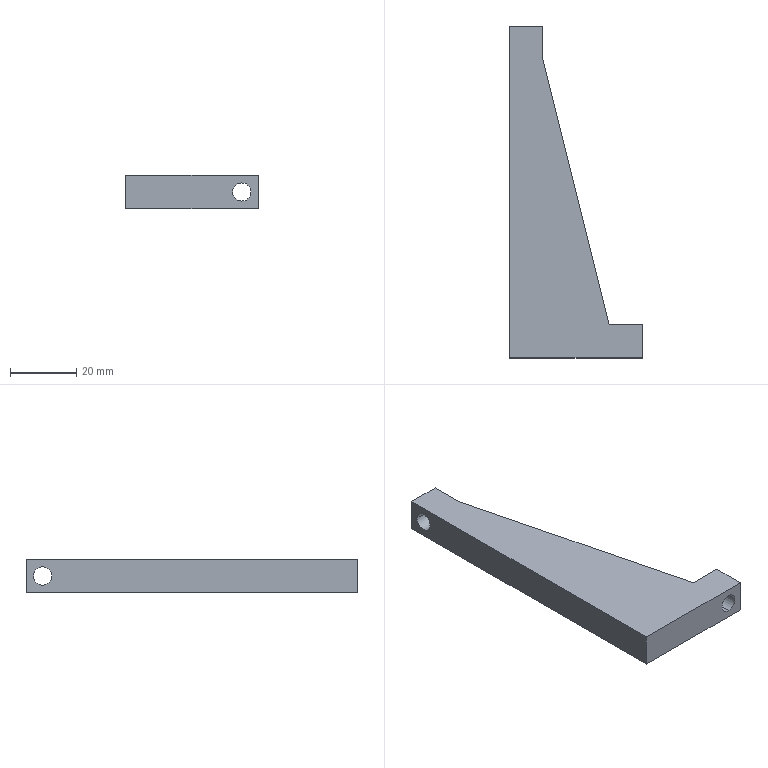Part | STEP file | B06 | 1 solid | 13 faces | box 40 x 100 x 10 mm | volume 20525 mm3 | plane 9 | cylinder 4 | commonest cylinder face diameters 5.5 x4
STEP:
#1=CARTESIAN_POINT('',(0.,0.,0.));
#2=DIRECTION('',(0.,0.,1.));
#3=DIRECTION('',(1.,0.,0.));
#4=AXIS2_PLACEMENT_3D('',#1,#2,#3);
#5=CARTESIAN_POINT('',(15.,-50.,7.75));
#6=VERTEX_POINT('',#5);
#7=CARTESIAN_POINT('',(15.,-40.,7.75));
#8=VERTEX_POINT('',#7);
#9=CARTESIAN_POINT('',(15.,-50.,7.75));
#10=DIRECTION('',(0.,1.,0.));
#11=VECTOR('',#10,1.);
#12=LINE('',#9,#11);
#13=CARTESIAN_POINT('',(15.,-50.,5.));
#14=DIRECTION('',(0.,1.,0.));
#15=DIRECTION('',(0.,0.,1.));
#16=AXIS2_PLACEMENT_3D('',#13,#14,#15);
#17=CYLINDRICAL_SURFACE('',#16,2.75);
#18=CARTESIAN_POINT('',(6.283,0.));
#19=DIRECTION('',(0.,1.));
#20=VECTOR('',#19,1.);
#21=LINE('',#18,#20);
#22=(GEOMETRIC_REPRESENTATION_CONTEXT(2)PARAMETRIC_REPRESENTATION_CONTEXT()REPRESENTATION_CONTEXT('',''));
#23=DEFINITIONAL_REPRESENTATION('',(#21),#22);
#24=PCURVE('',#17,#23);
#25=CARTESIAN_POINT('',(15.,-50.,5.));
#26=DIRECTION('',(0.,1.,0.));
#27=DIRECTION('',(0.,0.,1.));
#28=AXIS2_PLACEMENT_3D('',#25,#26,#27);
#29=CYLINDRICAL_SURFACE('',#28,2.75);
#30=CARTESIAN_POINT('',(0.,0.));
#31=DIRECTION('',(0.,1.));
#32=VECTOR('',#31,1.);
#33=LINE('',#30,#32);
#34=(GEOMETRIC_REPRESENTATION_CONTEXT(2)PARAMETRIC_REPRESENTATION_CONTEXT()REPRESENTATION_CONTEXT('',''));
#35=DEFINITIONAL_REPRESENTATION('',(#33),#34);
#36=PCURVE('',#29,#35);
#37=SURFACE_CURVE('',#12,(#24,#36),.PCURVE_S1.);
#38=EDGE_CURVE('',#6,#8,#37,.T.);
#39=ORIENTED_EDGE('',*,*,#38,.T.);
#40=CARTESIAN_POINT('',(15.,-40.,2.25));
#41=VERTEX_POINT('',#40);
#42=CARTESIAN_POINT('',(15.,-40.,5.));
#43=DIRECTION('',(0.,1.,0.));
#44=DIRECTION('',(0.,0.,1.));
#45=AXIS2_PLACEMENT_3D('',#42,#43,#44);
#46=CIRCLE('',#45,2.75);
#47=CARTESIAN_POINT('',(0.,10.));
#48=DIRECTION('',(1.,0.));
#49=VECTOR('',#48,1.);
#50=LINE('',#47,#49);
#51=(GEOMETRIC_REPRESENTATION_CONTEXT(2)PARAMETRIC_REPRESENTATION_CONTEXT()REPRESENTATION_CONTEXT('',''));
#52=DEFINITIONAL_REPRESENTATION('',(#50),#51);
#53=PCURVE('',#17,#52);
#54=CARTESIAN_POINT('',(10.,-40.,0.));
#55=DIRECTION('',(0.,-1.,0.));
#56=DIRECTION('',(0.,0.,-1.));
#57=AXIS2_PLACEMENT_3D('',#54,#55,#56);
#58=PLANE('',#57);
#59=CARTESIAN_POINT('',(-7.75,5.));
#60=CARTESIAN_POINT('',(-7.75,9.763));
#61=CARTESIAN_POINT('',(-3.625,7.382));
#62=CARTESIAN_POINT('',(0.5,5.));
#63=CARTESIAN_POINT('',(-3.625,2.618));
#64=CARTESIAN_POINT('',(-7.75,0.2369));
#65=CARTESIAN_POINT('',(-7.75,5.));
#66=(BOUNDED_CURVE()B_SPLINE_CURVE(2,(#59,#60,#61,#62,#63,#64,#65),.UNSPECIFIED.,.T.,.F.)B_SPLINE_CURVE_WITH_KNOTS((1,2,2,2,2,1),(-2.094,0.,2.094,4.189,6.283,8.378),.UNSPECIFIED.)CURVE()GEOMETRIC_REPRESENTATION_ITEM()RATIONAL_B_SPLINE_CURVE((1.,0.5,1.,0.5,1.,0.5,1.))REPRESENTATION_ITEM(''));
#67=(GEOMETRIC_REPRESENTATION_CONTEXT(2)PARAMETRIC_REPRESENTATION_CONTEXT()REPRESENTATION_CONTEXT('',''));
#68=DEFINITIONAL_REPRESENTATION('',(#66),#67);
#69=PCURVE('',#58,#68);
#70=SURFACE_CURVE('',#46,(#53,#69),.PCURVE_S1.);
#71=EDGE_CURVE('',#41,#8,#70,.T.);
#72=ORIENTED_EDGE('',*,*,#71,.F.);
#73=CARTESIAN_POINT('',(15.,-50.,2.25));
#74=VERTEX_POINT('',#73);
#75=CARTESIAN_POINT('',(15.,-50.,2.25));
#76=DIRECTION('',(0.,1.,0.));
#77=VECTOR('',#76,1.);
#78=LINE('',#75,#77);
#79=CARTESIAN_POINT('',(3.142,0.));
#80=DIRECTION('',(0.,1.));
#81=VECTOR('',#80,1.);
#82=LINE('',#79,#81);
#83=(GEOMETRIC_REPRESENTATION_CONTEXT(2)PARAMETRIC_REPRESENTATION_CONTEXT()REPRESENTATION_CONTEXT('',''));
#84=DEFINITIONAL_REPRESENTATION('',(#82),#83);
#85=PCURVE('',#17,#84);
#86=CARTESIAN_POINT('',(3.142,0.));
#87=DIRECTION('',(0.,1.));
#88=VECTOR('',#87,1.);
#89=LINE('',#86,#88);
#90=(GEOMETRIC_REPRESENTATION_CONTEXT(2)PARAMETRIC_REPRESENTATION_CONTEXT()REPRESENTATION_CONTEXT('',''));
#91=DEFINITIONAL_REPRESENTATION('',(#89),#90);
#92=PCURVE('',#29,#91);
#93=SURFACE_CURVE('',#78,(#85,#92),.PCURVE_S1.);
#94=EDGE_CURVE('',#74,#41,#93,.T.);
#95=ORIENTED_EDGE('',*,*,#94,.F.);
#96=CARTESIAN_POINT('',(15.,-50.,5.));
#97=DIRECTION('',(0.,1.,0.));
#98=DIRECTION('',(0.,0.,1.));
#99=AXIS2_PLACEMENT_3D('',#96,#97,#98);
#100=CIRCLE('',#99,2.75);
#101=CARTESIAN_POINT('',(0.,0.));
#102=DIRECTION('',(1.,0.));
#103=VECTOR('',#102,1.);
#104=LINE('',#101,#103);
#105=(GEOMETRIC_REPRESENTATION_CONTEXT(2)PARAMETRIC_REPRESENTATION_CONTEXT()REPRESENTATION_CONTEXT('',''));
#106=DEFINITIONAL_REPRESENTATION('',(#104),#105);
#107=PCURVE('',#17,#106);
#108=CARTESIAN_POINT('',(-20.,-50.,10.));
#109=DIRECTION('',(0.,1.,0.));
#110=DIRECTION('',(0.,0.,1.));
#111=AXIS2_PLACEMENT_3D('',#108,#109,#110);
#112=PLANE('',#111);
#113=CARTESIAN_POINT('',(-5.,35.));
#114=DIRECTION('',(1.,0.));
#115=AXIS2_PLACEMENT_2D('',#113,#114);
#116=CIRCLE('',#115,2.75);
#117=(GEOMETRIC_REPRESENTATION_CONTEXT(2)PARAMETRIC_REPRESENTATION_CONTEXT()REPRESENTATION_CONTEXT('',''));
#118=DEFINITIONAL_REPRESENTATION('',(#116),#117);
#119=PCURVE('',#112,#118);
#120=SURFACE_CURVE('',#100,(#107,#119),.PCURVE_S1.);
#121=EDGE_CURVE('',#74,#6,#120,.T.);
#122=ORIENTED_EDGE('',*,*,#121,.T.);
#123=EDGE_LOOP('',(#39,#72,#95,#122));
#124=FACE_BOUND('',#123,.F.);
#125=ADVANCED_FACE('',(#124),#17,.F.);
#126=CARTESIAN_POINT('',(-20.,47.75,5.));
#127=VERTEX_POINT('',#126);
#128=CARTESIAN_POINT('',(-10.,47.75,5.));
#129=VERTEX_POINT('',#128);
#130=CARTESIAN_POINT('',(-20.,47.75,5.));
#131=DIRECTION('',(1.,0.,0.));
#132=VECTOR('',#131,1.);
#133=LINE('',#130,#132);
#134=CARTESIAN_POINT('',(-20.,45.,5.));
#135=DIRECTION('',(1.,0.,0.));
#136=DIRECTION('',(0.,1.,0.));
#137=AXIS2_PLACEMENT_3D('',#134,#135,#136);
#138=CYLINDRICAL_SURFACE('',#137,2.75);
#139=CARTESIAN_POINT('',(6.283,0.));
#140=DIRECTION('',(0.,1.));
#141=VECTOR('',#140,1.);
#142=LINE('',#139,#141);
#143=(GEOMETRIC_REPRESENTATION_CONTEXT(2)PARAMETRIC_REPRESENTATION_CONTEXT()REPRESENTATION_CONTEXT('',''));
#144=DEFINITIONAL_REPRESENTATION('',(#142),#143);
#145=PCURVE('',#138,#144);
#146=CARTESIAN_POINT('',(-20.,45.,5.));
#147=DIRECTION('',(1.,0.,0.));
#148=DIRECTION('',(0.,1.,0.));
#149=AXIS2_PLACEMENT_3D('',#146,#147,#148);
#150=CYLINDRICAL_SURFACE('',#149,2.75);
#151=CARTESIAN_POINT('',(0.,0.));
#152=DIRECTION('',(0.,1.));
#153=VECTOR('',#152,1.);
#154=LINE('',#151,#153);
#155=(GEOMETRIC_REPRESENTATION_CONTEXT(2)PARAMETRIC_REPRESENTATION_CONTEXT()REPRESENTATION_CONTEXT('',''));
#156=DEFINITIONAL_REPRESENTATION('',(#154),#155);
#157=PCURVE('',#150,#156);
#158=SURFACE_CURVE('',#133,(#145,#157),.PCURVE_S1.);
#159=EDGE_CURVE('',#127,#129,#158,.T.);
#160=ORIENTED_EDGE('',*,*,#159,.T.);
#161=CARTESIAN_POINT('',(-10.,42.25,5.));
#162=VERTEX_POINT('',#161);
#163=CARTESIAN_POINT('',(-10.,45.,5.));
#164=DIRECTION('',(1.,0.,0.));
#165=DIRECTION('',(0.,1.,0.));
#166=AXIS2_PLACEMENT_3D('',#163,#164,#165);
#167=CIRCLE('',#166,2.75);
#168=CARTESIAN_POINT('',(0.,10.));
#169=DIRECTION('',(1.,0.));
#170=VECTOR('',#169,1.);
#171=LINE('',#168,#170);
#172=(GEOMETRIC_REPRESENTATION_CONTEXT(2)PARAMETRIC_REPRESENTATION_CONTEXT()REPRESENTATION_CONTEXT('',''));
#173=DEFINITIONAL_REPRESENTATION('',(#171),#172);
#174=PCURVE('',#138,#173);
#175=CARTESIAN_POINT('',(-10.,50.,0.));
#176=DIRECTION('',(-1.,0.,0.));
#177=DIRECTION('',(0.,-1.,0.));
#178=AXIS2_PLACEMENT_3D('',#175,#176,#177);
#179=PLANE('',#178);
#180=CARTESIAN_POINT('',(2.25,5.));
#181=CARTESIAN_POINT('',(2.25,9.763));
#182=CARTESIAN_POINT('',(6.375,7.382));
#183=CARTESIAN_POINT('',(10.5,5.));
#184=CARTESIAN_POINT('',(6.375,2.618));
#185=CARTESIAN_POINT('',(2.25,0.2369));
#186=CARTESIAN_POINT('',(2.25,5.));
#187=(BOUNDED_CURVE()B_SPLINE_CURVE(2,(#180,#181,#182,#183,#184,#185,#186),.UNSPECIFIED.,.T.,.F.)B_SPLINE_CURVE_WITH_KNOTS((1,2,2,2,2,1),(-2.094,0.,2.094,4.189,6.283,8.378),.UNSPECIFIED.)CURVE()GEOMETRIC_REPRESENTATION_ITEM()RATIONAL_B_SPLINE_CURVE((1.,0.5,1.,0.5,1.,0.5,1.))REPRESENTATION_ITEM(''));
#188=(GEOMETRIC_REPRESENTATION_CONTEXT(2)PARAMETRIC_REPRESENTATION_CONTEXT()REPRESENTATION_CONTEXT('',''));
#189=DEFINITIONAL_REPRESENTATION('',(#187),#188);
#190=PCURVE('',#179,#189);
#191=SURFACE_CURVE('',#167,(#174,#190),.PCURVE_S1.);
#192=EDGE_CURVE('',#162,#129,#191,.T.);
#193=ORIENTED_EDGE('',*,*,#192,.F.);
#194=CARTESIAN_POINT('',(-20.,42.25,5.));
#195=VERTEX_POINT('',#194);
#196=CARTESIAN_POINT('',(-20.,42.25,5.));
#197=DIRECTION('',(1.,0.,0.));
#198=VECTOR('',#197,1.);
#199=LINE('',#196,#198);
#200=CARTESIAN_POINT('',(3.142,0.));
#201=DIRECTION('',(0.,1.));
#202=VECTOR('',#201,1.);
#203=LINE('',#200,#202);
#204=(GEOMETRIC_REPRESENTATION_CONTEXT(2)PARAMETRIC_REPRESENTATION_CONTEXT()REPRESENTATION_CONTEXT('',''));
#205=DEFINITIONAL_REPRESENTATION('',(#203),#204);
#206=PCURVE('',#138,#205);
#207=CARTESIAN_POINT('',(3.142,0.));
#208=DIRECTION('',(0.,1.));
#209=VECTOR('',#208,1.);
#210=LINE('',#207,#209);
#211=(GEOMETRIC_REPRESENTATION_CONTEXT(2)PARAMETRIC_REPRESENTATION_CONTEXT()REPRESENTATION_CONTEXT('',''));
#212=DEFINITIONAL_REPRESENTATION('',(#210),#211);
#213=PCURVE('',#150,#212);
#214=SURFACE_CURVE('',#199,(#206,#213),.PCURVE_S1.);
#215=EDGE_CURVE('',#195,#162,#214,.T.);
#216=ORIENTED_EDGE('',*,*,#215,.F.);
#217=CARTESIAN_POINT('',(-20.,45.,5.));
#218=DIRECTION('',(1.,0.,0.));
#219=DIRECTION('',(0.,1.,0.));
#220=AXIS2_PLACEMENT_3D('',#217,#218,#219);
#221=CIRCLE('',#220,2.75);
#222=CARTESIAN_POINT('',(0.,0.));
#223=DIRECTION('',(1.,0.));
#224=VECTOR('',#223,1.);
#225=LINE('',#222,#224);
#226=(GEOMETRIC_REPRESENTATION_CONTEXT(2)PARAMETRIC_REPRESENTATION_CONTEXT()REPRESENTATION_CONTEXT('',''));
#227=DEFINITIONAL_REPRESENTATION('',(#225),#226);
#228=PCURVE('',#138,#227);
#229=CARTESIAN_POINT('',(-20.,50.,10.));
#230=DIRECTION('',(1.,0.,0.));
#231=DIRECTION('',(0.,1.,0.));
#232=AXIS2_PLACEMENT_3D('',#229,#230,#231);
#233=PLANE('',#232);
#234=CARTESIAN_POINT('',(-5.,-5.));
#235=DIRECTION('',(1.,0.));
#236=AXIS2_PLACEMENT_2D('',#234,#235);
#237=CIRCLE('',#236,2.75);
#238=(GEOMETRIC_REPRESENTATION_CONTEXT(2)PARAMETRIC_REPRESENTATION_CONTEXT()REPRESENTATION_CONTEXT('',''));
#239=DEFINITIONAL_REPRESENTATION('',(#237),#238);
#240=PCURVE('',#233,#239);
#241=SURFACE_CURVE('',#221,(#228,#240),.PCURVE_S1.);
#242=EDGE_CURVE('',#195,#127,#241,.T.);
#243=ORIENTED_EDGE('',*,*,#242,.T.);
#244=EDGE_LOOP('',(#160,#193,#216,#243));
#245=FACE_BOUND('',#244,.F.);
#246=ADVANCED_FACE('',(#245),#138,.F.);
#247=CARTESIAN_POINT('',(20.,-50.,0.));
#248=VERTEX_POINT('',#247);
#249=CARTESIAN_POINT('',(20.,-40.,0.));
#250=VERTEX_POINT('',#249);
#251=CARTESIAN_POINT('',(20.,50.,0.));
#252=DIRECTION('',(0.,1.,0.));
#253=VECTOR('',#252,1.);
#254=LINE('',#251,#253);
#255=CARTESIAN_POINT('',(20.,50.,10.));
#256=DIRECTION('',(-1.,0.,0.));
#257=DIRECTION('',(0.,-1.,0.));
#258=AXIS2_PLACEMENT_3D('',#255,#256,#257);
#259=PLANE('',#258);
#260=CARTESIAN_POINT('',(0.,-10.));
#261=DIRECTION('',(-1.,0.));
#262=VECTOR('',#261,1.);
#263=LINE('',#260,#262);
#264=(GEOMETRIC_REPRESENTATION_CONTEXT(2)PARAMETRIC_REPRESENTATION_CONTEXT()REPRESENTATION_CONTEXT('',''));
#265=DEFINITIONAL_REPRESENTATION('',(#263),#264);
#266=PCURVE('',#259,#265);
#267=CARTESIAN_POINT('',(0.,0.,0.));
#268=DIRECTION('',(0.,0.,1.));
#269=DIRECTION('',(1.,0.,0.));
#270=AXIS2_PLACEMENT_3D('',#267,#268,#269);
#271=PLANE('',#270);
#272=CARTESIAN_POINT('',(20.,50.));
#273=DIRECTION('',(0.,1.));
#274=VECTOR('',#273,1.);
#275=LINE('',#272,#274);
#276=(GEOMETRIC_REPRESENTATION_CONTEXT(2)PARAMETRIC_REPRESENTATION_CONTEXT()REPRESENTATION_CONTEXT('',''));
#277=DEFINITIONAL_REPRESENTATION('',(#275),#276);
#278=PCURVE('',#271,#277);
#279=SURFACE_CURVE('',#254,(#266,#278),.PCURVE_S1.);
#280=EDGE_CURVE('',#248,#250,#279,.T.);
#281=ORIENTED_EDGE('',*,*,#280,.T.);
#282=CARTESIAN_POINT('',(20.,-40.,10.));
#283=VERTEX_POINT('',#282);
#284=CARTESIAN_POINT('',(20.,-40.,0.));
#285=DIRECTION('',(0.,0.,1.));
#286=VECTOR('',#285,1.);
#287=LINE('',#284,#286);
#288=CARTESIAN_POINT('',(90.,-10.));
#289=DIRECTION('',(0.,1.));
#290=VECTOR('',#289,1.);
#291=LINE('',#288,#290);
#292=(GEOMETRIC_REPRESENTATION_CONTEXT(2)PARAMETRIC_REPRESENTATION_CONTEXT()REPRESENTATION_CONTEXT('',''));
#293=DEFINITIONAL_REPRESENTATION('',(#291),#292);
#294=PCURVE('',#259,#293);
#295=CARTESIAN_POINT('',(0.,10.));
#296=DIRECTION('',(-1.,0.));
#297=VECTOR('',#296,1.);
#298=LINE('',#295,#297);
#299=(GEOMETRIC_REPRESENTATION_CONTEXT(2)PARAMETRIC_REPRESENTATION_CONTEXT()REPRESENTATION_CONTEXT('',''));
#300=DEFINITIONAL_REPRESENTATION('',(#298),#299);
#301=PCURVE('',#58,#300);
#302=SURFACE_CURVE('',#287,(#294,#301),.PCURVE_S1.);
#303=EDGE_CURVE('',#250,#283,#302,.T.);
#304=ORIENTED_EDGE('',*,*,#303,.T.);
#305=CARTESIAN_POINT('',(20.,-50.,10.));
#306=VERTEX_POINT('',#305);
#307=CARTESIAN_POINT('',(20.,50.,10.));
#308=DIRECTION('',(0.,1.,0.));
#309=VECTOR('',#308,1.);
#310=LINE('',#307,#309);
#311=CARTESIAN_POINT('',(0.,0.));
#312=DIRECTION('',(-1.,0.));
#313=VECTOR('',#312,1.);
#314=LINE('',#311,#313);
#315=(GEOMETRIC_REPRESENTATION_CONTEXT(2)PARAMETRIC_REPRESENTATION_CONTEXT()REPRESENTATION_CONTEXT('',''));
#316=DEFINITIONAL_REPRESENTATION('',(#314),#315);
#317=PCURVE('',#259,#316);
#318=CARTESIAN_POINT('',(0.,0.,10.));
#319=DIRECTION('',(0.,0.,1.));
#320=DIRECTION('',(1.,0.,0.));
#321=AXIS2_PLACEMENT_3D('',#318,#319,#320);
#322=PLANE('',#321);
#323=CARTESIAN_POINT('',(20.,50.));
#324=DIRECTION('',(0.,1.));
#325=VECTOR('',#324,1.);
#326=LINE('',#323,#325);
#327=(GEOMETRIC_REPRESENTATION_CONTEXT(2)PARAMETRIC_REPRESENTATION_CONTEXT()REPRESENTATION_CONTEXT('',''));
#328=DEFINITIONAL_REPRESENTATION('',(#326),#327);
#329=PCURVE('',#322,#328);
#330=SURFACE_CURVE('',#310,(#317,#329),.PCURVE_S1.);
#331=EDGE_CURVE('',#306,#283,#330,.T.);
#332=ORIENTED_EDGE('',*,*,#331,.F.);
#333=CARTESIAN_POINT('',(20.,-50.,10.));
#334=DIRECTION('',(0.,0.,-1.));
#335=VECTOR('',#334,1.);
#336=LINE('',#333,#335);
#337=CARTESIAN_POINT('',(100.,0.));
#338=DIRECTION('',(0.,-1.));
#339=VECTOR('',#338,1.);
#340=LINE('',#337,#339);
#341=(GEOMETRIC_REPRESENTATION_CONTEXT(2)PARAMETRIC_REPRESENTATION_CONTEXT()REPRESENTATION_CONTEXT('',''));
#342=DEFINITIONAL_REPRESENTATION('',(#340),#341);
#343=PCURVE('',#259,#342);
#344=CARTESIAN_POINT('',(0.,40.));
#345=DIRECTION('',(-1.,0.));
#346=VECTOR('',#345,1.);
#347=LINE('',#344,#346);
#348=(GEOMETRIC_REPRESENTATION_CONTEXT(2)PARAMETRIC_REPRESENTATION_CONTEXT()REPRESENTATION_CONTEXT('',''));
#349=DEFINITIONAL_REPRESENTATION('',(#347),#348);
#350=PCURVE('',#112,#349);
#351=SURFACE_CURVE('',#336,(#343,#350),.PCURVE_S1.);
#352=EDGE_CURVE('',#306,#248,#351,.T.);
#353=ORIENTED_EDGE('',*,*,#352,.T.);
#354=EDGE_LOOP('',(#281,#304,#332,#353));
#355=FACE_BOUND('',#354,.T.);
#356=ADVANCED_FACE('',(#355),#259,.F.);
#357=CARTESIAN_POINT('',(-10.,50.,10.));
#358=VERTEX_POINT('',#357);
#359=CARTESIAN_POINT('',(-20.,50.,10.));
#360=VERTEX_POINT('',#359);
#361=CARTESIAN_POINT('',(-20.,50.,10.));
#362=DIRECTION('',(-1.,0.,0.));
#363=VECTOR('',#362,1.);
#364=LINE('',#361,#363);
#365=CARTESIAN_POINT('',(-20.,50.,10.));
#366=DIRECTION('',(0.,-1.,0.));
#367=DIRECTION('',(0.,0.,-1.));
#368=AXIS2_PLACEMENT_3D('',#365,#366,#367);
#369=PLANE('',#368);
#370=CARTESIAN_POINT('',(0.,0.));
#371=DIRECTION('',(0.,-1.));
#372=VECTOR('',#371,1.);
#373=LINE('',#370,#372);
#374=(GEOMETRIC_REPRESENTATION_CONTEXT(2)PARAMETRIC_REPRESENTATION_CONTEXT()REPRESENTATION_CONTEXT('',''));
#375=DEFINITIONAL_REPRESENTATION('',(#373),#374);
#376=PCURVE('',#369,#375);
#377=CARTESIAN_POINT('',(-20.,50.));
#378=DIRECTION('',(-1.,0.));
#379=VECTOR('',#378,1.);
#380=LINE('',#377,#379);
#381=(GEOMETRIC_REPRESENTATION_CONTEXT(2)PARAMETRIC_REPRESENTATION_CONTEXT()REPRESENTATION_CONTEXT('',''));
#382=DEFINITIONAL_REPRESENTATION('',(#380),#381);
#383=PCURVE('',#322,#382);
#384=SURFACE_CURVE('',#364,(#376,#383),.PCURVE_S1.);
#385=EDGE_CURVE('',#358,#360,#384,.T.);
#386=ORIENTED_EDGE('',*,*,#385,.F.);
#387=CARTESIAN_POINT('',(-10.,50.,0.));
#388=VERTEX_POINT('',#387);
#389=CARTESIAN_POINT('',(-10.,50.,0.));
#390=DIRECTION('',(0.,0.,1.));
#391=VECTOR('',#390,1.);
#392=LINE('',#389,#391);
#393=CARTESIAN_POINT('',(10.,10.));
#394=DIRECTION('',(-1.,0.));
#395=VECTOR('',#394,1.);
#396=LINE('',#393,#395);
#397=(GEOMETRIC_REPRESENTATION_CONTEXT(2)PARAMETRIC_REPRESENTATION_CONTEXT()REPRESENTATION_CONTEXT('',''));
#398=DEFINITIONAL_REPRESENTATION('',(#396),#397);
#399=PCURVE('',#369,#398);
#400=CARTESIAN_POINT('',(0.,0.));
#401=DIRECTION('',(0.,1.));
#402=VECTOR('',#401,1.);
#403=LINE('',#400,#402);
#404=(GEOMETRIC_REPRESENTATION_CONTEXT(2)PARAMETRIC_REPRESENTATION_CONTEXT()REPRESENTATION_CONTEXT('',''));
#405=DEFINITIONAL_REPRESENTATION('',(#403),#404);
#406=PCURVE('',#179,#405);
#407=SURFACE_CURVE('',#392,(#399,#406),.PCURVE_S1.);
#408=EDGE_CURVE('',#388,#358,#407,.T.);
#409=ORIENTED_EDGE('',*,*,#408,.F.);
#410=CARTESIAN_POINT('',(-20.,50.,0.));
#411=VERTEX_POINT('',#410);
#412=CARTESIAN_POINT('',(-20.,50.,0.));
#413=DIRECTION('',(-1.,0.,0.));
#414=VECTOR('',#413,1.);
#415=LINE('',#412,#414);
#416=CARTESIAN_POINT('',(10.,0.));
#417=DIRECTION('',(0.,-1.));
#418=VECTOR('',#417,1.);
#419=LINE('',#416,#418);
#420=(GEOMETRIC_REPRESENTATION_CONTEXT(2)PARAMETRIC_REPRESENTATION_CONTEXT()REPRESENTATION_CONTEXT('',''));
#421=DEFINITIONAL_REPRESENTATION('',(#419),#420);
#422=PCURVE('',#369,#421);
#423=CARTESIAN_POINT('',(-20.,50.));
#424=DIRECTION('',(-1.,0.));
#425=VECTOR('',#424,1.);
#426=LINE('',#423,#425);
#427=(GEOMETRIC_REPRESENTATION_CONTEXT(2)PARAMETRIC_REPRESENTATION_CONTEXT()REPRESENTATION_CONTEXT('',''));
#428=DEFINITIONAL_REPRESENTATION('',(#426),#427);
#429=PCURVE('',#271,#428);
#430=SURFACE_CURVE('',#415,(#422,#429),.PCURVE_S1.);
#431=EDGE_CURVE('',#388,#411,#430,.T.);
#432=ORIENTED_EDGE('',*,*,#431,.T.);
#433=CARTESIAN_POINT('',(-20.,50.,10.));
#434=DIRECTION('',(0.,0.,-1.));
#435=VECTOR('',#434,1.);
#436=LINE('',#433,#435);
#437=CARTESIAN_POINT('',(0.,0.));
#438=DIRECTION('',(1.,0.));
#439=VECTOR('',#438,1.);
#440=LINE('',#437,#439);
#441=(GEOMETRIC_REPRESENTATION_CONTEXT(2)PARAMETRIC_REPRESENTATION_CONTEXT()REPRESENTATION_CONTEXT('',''));
#442=DEFINITIONAL_REPRESENTATION('',(#440),#441);
#443=PCURVE('',#369,#442);
#444=CARTESIAN_POINT('',(0.,0.));
#445=DIRECTION('',(0.,-1.));
#446=VECTOR('',#445,1.);
#447=LINE('',#444,#446);
#448=(GEOMETRIC_REPRESENTATION_CONTEXT(2)PARAMETRIC_REPRESENTATION_CONTEXT()REPRESENTATION_CONTEXT('',''));
#449=DEFINITIONAL_REPRESENTATION('',(#447),#448);
#450=PCURVE('',#233,#449);
#451=SURFACE_CURVE('',#436,(#443,#450),.PCURVE_S1.);
#452=EDGE_CURVE('',#360,#411,#451,.T.);
#453=ORIENTED_EDGE('',*,*,#452,.F.);
#454=EDGE_LOOP('',(#386,#409,#432,#453));
#455=FACE_BOUND('',#454,.T.);
#456=ADVANCED_FACE('',(#455),#369,.F.);
#457=CARTESIAN_POINT('',(-20.,45.,5.));
#458=DIRECTION('',(1.,0.,0.));
#459=DIRECTION('',(0.,1.,0.));
#460=AXIS2_PLACEMENT_3D('',#457,#458,#459);
#461=CIRCLE('',#460,2.75);
#462=CARTESIAN_POINT('',(-5.,-5.));
#463=DIRECTION('',(1.,0.));
#464=AXIS2_PLACEMENT_2D('',#462,#463);
#465=CIRCLE('',#464,2.75);
#466=(GEOMETRIC_REPRESENTATION_CONTEXT(2)PARAMETRIC_REPRESENTATION_CONTEXT()REPRESENTATION_CONTEXT('',''));
#467=DEFINITIONAL_REPRESENTATION('',(#465),#466);
#468=PCURVE('',#233,#467);
#469=CARTESIAN_POINT('',(0.,0.));
#470=DIRECTION('',(1.,0.));
#471=VECTOR('',#470,1.);
#472=LINE('',#469,#471);
#473=(GEOMETRIC_REPRESENTATION_CONTEXT(2)PARAMETRIC_REPRESENTATION_CONTEXT()REPRESENTATION_CONTEXT('',''));
#474=DEFINITIONAL_REPRESENTATION('',(#472),#473);
#475=PCURVE('',#150,#474);
#476=SURFACE_CURVE('',#461,(#468,#475),.PCURVE_S1.);
#477=EDGE_CURVE('',#127,#195,#476,.T.);
#478=ORIENTED_EDGE('',*,*,#477,.T.);
#479=ORIENTED_EDGE('',*,*,#242,.T.);
#480=EDGE_LOOP('',(#478,#479));
#481=FACE_BOUND('',#480,.T.);
#482=CARTESIAN_POINT('',(-20.,-50.,0.));
#483=VERTEX_POINT('',#482);
#484=CARTESIAN_POINT('',(-20.,50.,0.));
#485=DIRECTION('',(0.,-1.,0.));
#486=VECTOR('',#485,1.);
#487=LINE('',#484,#486);
#488=CARTESIAN_POINT('',(0.,-10.));
#489=DIRECTION('',(-1.,0.));
#490=VECTOR('',#489,1.);
#491=LINE('',#488,#490);
#492=(GEOMETRIC_REPRESENTATION_CONTEXT(2)PARAMETRIC_REPRESENTATION_CONTEXT()REPRESENTATION_CONTEXT('',''));
#493=DEFINITIONAL_REPRESENTATION('',(#491),#492);
#494=PCURVE('',#233,#493);
#495=CARTESIAN_POINT('',(-20.,50.));
#496=DIRECTION('',(0.,-1.));
#497=VECTOR('',#496,1.);
#498=LINE('',#495,#497);
#499=(GEOMETRIC_REPRESENTATION_CONTEXT(2)PARAMETRIC_REPRESENTATION_CONTEXT()REPRESENTATION_CONTEXT('',''));
#500=DEFINITIONAL_REPRESENTATION('',(#498),#499);
#501=PCURVE('',#271,#500);
#502=SURFACE_CURVE('',#487,(#494,#501),.PCURVE_S1.);
#503=EDGE_CURVE('',#411,#483,#502,.T.);
#504=ORIENTED_EDGE('',*,*,#503,.T.);
#505=CARTESIAN_POINT('',(-20.,-50.,10.));
#506=VERTEX_POINT('',#505);
#507=CARTESIAN_POINT('',(-20.,-50.,10.));
#508=DIRECTION('',(0.,0.,-1.));
#509=VECTOR('',#508,1.);
#510=LINE('',#507,#509);
#511=CARTESIAN_POINT('',(-100.,0.));
#512=DIRECTION('',(0.,-1.));
#513=VECTOR('',#512,1.);
#514=LINE('',#511,#513);
#515=(GEOMETRIC_REPRESENTATION_CONTEXT(2)PARAMETRIC_REPRESENTATION_CONTEXT()REPRESENTATION_CONTEXT('',''));
#516=DEFINITIONAL_REPRESENTATION('',(#514),#515);
#517=PCURVE('',#233,#516);
#518=CARTESIAN_POINT('',(0.,0.));
#519=DIRECTION('',(-1.,0.));
#520=VECTOR('',#519,1.);
#521=LINE('',#518,#520);
#522=(GEOMETRIC_REPRESENTATION_CONTEXT(2)PARAMETRIC_REPRESENTATION_CONTEXT()REPRESENTATION_CONTEXT('',''));
#523=DEFINITIONAL_REPRESENTATION('',(#521),#522);
#524=PCURVE('',#112,#523);
#525=SURFACE_CURVE('',#510,(#517,#524),.PCURVE_S1.);
#526=EDGE_CURVE('',#506,#483,#525,.T.);
#527=ORIENTED_EDGE('',*,*,#526,.F.);
#528=CARTESIAN_POINT('',(-20.,50.,10.));
#529=DIRECTION('',(0.,-1.,0.));
#530=VECTOR('',#529,1.);
#531=LINE('',#528,#530);
#532=CARTESIAN_POINT('',(0.,0.));
#533=DIRECTION('',(-1.,0.));
#534=VECTOR('',#533,1.);
#535=LINE('',#532,#534);
#536=(GEOMETRIC_REPRESENTATION_CONTEXT(2)PARAMETRIC_REPRESENTATION_CONTEXT()REPRESENTATION_CONTEXT('',''));
#537=DEFINITIONAL_REPRESENTATION('',(#535),#536);
#538=PCURVE('',#233,#537);
#539=CARTESIAN_POINT('',(-20.,50.));
#540=DIRECTION('',(0.,-1.));
#541=VECTOR('',#540,1.);
#542=LINE('',#539,#541);
#543=(GEOMETRIC_REPRESENTATION_CONTEXT(2)PARAMETRIC_REPRESENTATION_CONTEXT()REPRESENTATION_CONTEXT('',''));
#544=DEFINITIONAL_REPRESENTATION('',(#542),#543);
#545=PCURVE('',#322,#544);
#546=SURFACE_CURVE('',#531,(#538,#545),.PCURVE_S1.);
#547=EDGE_CURVE('',#360,#506,#546,.T.);
#548=ORIENTED_EDGE('',*,*,#547,.F.);
#549=ORIENTED_EDGE('',*,*,#452,.T.);
#550=EDGE_LOOP('',(#504,#527,#548,#549));
#551=FACE_BOUND('',#550,.T.);
#552=ADVANCED_FACE('',(#481,#551),#233,.F.);
#553=CARTESIAN_POINT('',(15.,-50.,5.));
#554=DIRECTION('',(0.,1.,0.));
#555=DIRECTION('',(0.,0.,1.));
#556=AXIS2_PLACEMENT_3D('',#553,#554,#555);
#557=CIRCLE('',#556,2.75);
#558=CARTESIAN_POINT('',(-5.,35.));
#559=DIRECTION('',(1.,0.));
#560=AXIS2_PLACEMENT_2D('',#558,#559);
#561=CIRCLE('',#560,2.75);
#562=(GEOMETRIC_REPRESENTATION_CONTEXT(2)PARAMETRIC_REPRESENTATION_CONTEXT()REPRESENTATION_CONTEXT('',''));
#563=DEFINITIONAL_REPRESENTATION('',(#561),#562);
#564=PCURVE('',#112,#563);
#565=CARTESIAN_POINT('',(0.,0.));
#566=DIRECTION('',(1.,0.));
#567=VECTOR('',#566,1.);
#568=LINE('',#565,#567);
#569=(GEOMETRIC_REPRESENTATION_CONTEXT(2)PARAMETRIC_REPRESENTATION_CONTEXT()REPRESENTATION_CONTEXT('',''));
#570=DEFINITIONAL_REPRESENTATION('',(#568),#569);
#571=PCURVE('',#29,#570);
#572=SURFACE_CURVE('',#557,(#564,#571),.PCURVE_S1.);
#573=EDGE_CURVE('',#6,#74,#572,.T.);
#574=ORIENTED_EDGE('',*,*,#573,.T.);
#575=ORIENTED_EDGE('',*,*,#121,.T.);
#576=EDGE_LOOP('',(#574,#575));
#577=FACE_BOUND('',#576,.T.);
#578=CARTESIAN_POINT('',(-20.,-50.,0.));
#579=DIRECTION('',(1.,0.,0.));
#580=VECTOR('',#579,1.);
#581=LINE('',#578,#580);
#582=CARTESIAN_POINT('',(-10.,0.));
#583=DIRECTION('',(0.,1.));
#584=VECTOR('',#583,1.);
#585=LINE('',#582,#584);
#586=(GEOMETRIC_REPRESENTATION_CONTEXT(2)PARAMETRIC_REPRESENTATION_CONTEXT()REPRESENTATION_CONTEXT('',''));
#587=DEFINITIONAL_REPRESENTATION('',(#585),#586);
#588=PCURVE('',#112,#587);
#589=CARTESIAN_POINT('',(-20.,-50.));
#590=DIRECTION('',(1.,0.));
#591=VECTOR('',#590,1.);
#592=LINE('',#589,#591);
#593=(GEOMETRIC_REPRESENTATION_CONTEXT(2)PARAMETRIC_REPRESENTATION_CONTEXT()REPRESENTATION_CONTEXT('',''));
#594=DEFINITIONAL_REPRESENTATION('',(#592),#593);
#595=PCURVE('',#271,#594);
#596=SURFACE_CURVE('',#581,(#588,#595),.PCURVE_S1.);
#597=EDGE_CURVE('',#483,#248,#596,.T.);
#598=ORIENTED_EDGE('',*,*,#597,.T.);
#599=ORIENTED_EDGE('',*,*,#352,.F.);
#600=CARTESIAN_POINT('',(-20.,-50.,10.));
#601=DIRECTION('',(1.,0.,0.));
#602=VECTOR('',#601,1.);
#603=LINE('',#600,#602);
#604=CARTESIAN_POINT('',(0.,0.));
#605=DIRECTION('',(0.,1.));
#606=VECTOR('',#605,1.);
#607=LINE('',#604,#606);
#608=(GEOMETRIC_REPRESENTATION_CONTEXT(2)PARAMETRIC_REPRESENTATION_CONTEXT()REPRESENTATION_CONTEXT('',''));
#609=DEFINITIONAL_REPRESENTATION('',(#607),#608);
#610=PCURVE('',#112,#609);
#611=CARTESIAN_POINT('',(-20.,-50.));
#612=DIRECTION('',(1.,0.));
#613=VECTOR('',#612,1.);
#614=LINE('',#611,#613);
#615=(GEOMETRIC_REPRESENTATION_CONTEXT(2)PARAMETRIC_REPRESENTATION_CONTEXT()REPRESENTATION_CONTEXT('',''));
#616=DEFINITIONAL_REPRESENTATION('',(#614),#615);
#617=PCURVE('',#322,#616);
#618=SURFACE_CURVE('',#603,(#610,#617),.PCURVE_S1.);
#619=EDGE_CURVE('',#506,#306,#618,.T.);
#620=ORIENTED_EDGE('',*,*,#619,.F.);
#621=ORIENTED_EDGE('',*,*,#526,.T.);
#622=EDGE_LOOP('',(#598,#599,#620,#621));
#623=FACE_BOUND('',#622,.T.);
#624=ADVANCED_FACE('',(#577,#623),#112,.F.);
#625=CARTESIAN_POINT('',(10.,-40.,10.));
#626=VERTEX_POINT('',#625);
#627=CARTESIAN_POINT('',(10.,-40.,10.));
#628=DIRECTION('',(1.,0.,0.));
#629=VECTOR('',#628,1.);
#630=LINE('',#627,#629);
#631=CARTESIAN_POINT('',(10.,-40.));
#632=DIRECTION('',(1.,0.));
#633=VECTOR('',#632,1.);
#634=LINE('',#631,#633);
#635=(GEOMETRIC_REPRESENTATION_CONTEXT(2)PARAMETRIC_REPRESENTATION_CONTEXT()REPRESENTATION_CONTEXT('',''));
#636=DEFINITIONAL_REPRESENTATION('',(#634),#635);
#637=PCURVE('',#322,#636);
#638=CARTESIAN_POINT('',(-10.,0.));
#639=DIRECTION('',(0.,1.));
#640=VECTOR('',#639,1.);
#641=LINE('',#638,#640);
#642=(GEOMETRIC_REPRESENTATION_CONTEXT(2)PARAMETRIC_REPRESENTATION_CONTEXT()REPRESENTATION_CONTEXT('',''));
#643=DEFINITIONAL_REPRESENTATION('',(#641),#642);
#644=PCURVE('',#58,#643);
#645=SURFACE_CURVE('',#630,(#637,#644),.PCURVE_S1.);
#646=EDGE_CURVE('',#626,#283,#645,.T.);
#647=ORIENTED_EDGE('',*,*,#646,.F.);
#648=CARTESIAN_POINT('',(-10.,40.,10.));
#649=VERTEX_POINT('',#648);
#650=CARTESIAN_POINT('',(-10.,40.,10.));
#651=DIRECTION('',(0.2425,-0.9701,0.));
#652=VECTOR('',#651,1.);
#653=LINE('',#650,#652);
#654=CARTESIAN_POINT('',(-10.,40.));
#655=DIRECTION('',(0.2425,-0.9701));
#656=VECTOR('',#655,1.);
#657=LINE('',#654,#656);
#658=(GEOMETRIC_REPRESENTATION_CONTEXT(2)PARAMETRIC_REPRESENTATION_CONTEXT()REPRESENTATION_CONTEXT('',''));
#659=DEFINITIONAL_REPRESENTATION('',(#657),#658);
#660=PCURVE('',#322,#659);
#661=CARTESIAN_POINT('',(-10.,40.,0.));
#662=DIRECTION('',(-0.9701,-0.2425,0.));
#663=DIRECTION('',(0.2425,-0.9701,0.));
#664=AXIS2_PLACEMENT_3D('',#661,#662,#663);
#665=PLANE('',#664);
#666=CARTESIAN_POINT('',(0.,10.));
#667=DIRECTION('',(1.,0.));
#668=VECTOR('',#667,1.);
#669=LINE('',#666,#668);
#670=(GEOMETRIC_REPRESENTATION_CONTEXT(2)PARAMETRIC_REPRESENTATION_CONTEXT()REPRESENTATION_CONTEXT('',''));
#671=DEFINITIONAL_REPRESENTATION('',(#669),#670);
#672=PCURVE('',#665,#671);
#673=SURFACE_CURVE('',#653,(#660,#672),.PCURVE_S1.);
#674=EDGE_CURVE('',#649,#626,#673,.T.);
#675=ORIENTED_EDGE('',*,*,#674,.F.);
#676=CARTESIAN_POINT('',(-10.,50.,10.));
#677=DIRECTION('',(0.,-1.,0.));
#678=VECTOR('',#677,1.);
#679=LINE('',#676,#678);
#680=CARTESIAN_POINT('',(-10.,50.));
#681=DIRECTION('',(0.,-1.));
#682=VECTOR('',#681,1.);
#683=LINE('',#680,#682);
#684=(GEOMETRIC_REPRESENTATION_CONTEXT(2)PARAMETRIC_REPRESENTATION_CONTEXT()REPRESENTATION_CONTEXT('',''));
#685=DEFINITIONAL_REPRESENTATION('',(#683),#684);
#686=PCURVE('',#322,#685);
#687=CARTESIAN_POINT('',(0.,10.));
#688=DIRECTION('',(1.,0.));
#689=VECTOR('',#688,1.);
#690=LINE('',#687,#689);
#691=(GEOMETRIC_REPRESENTATION_CONTEXT(2)PARAMETRIC_REPRESENTATION_CONTEXT()REPRESENTATION_CONTEXT('',''));
#692=DEFINITIONAL_REPRESENTATION('',(#690),#691);
#693=PCURVE('',#179,#692);
#694=SURFACE_CURVE('',#679,(#686,#693),.PCURVE_S1.);
#695=EDGE_CURVE('',#358,#649,#694,.T.);
#696=ORIENTED_EDGE('',*,*,#695,.F.);
#697=ORIENTED_EDGE('',*,*,#385,.T.);
#698=ORIENTED_EDGE('',*,*,#547,.T.);
#699=ORIENTED_EDGE('',*,*,#619,.T.);
#700=ORIENTED_EDGE('',*,*,#331,.T.);
#701=EDGE_LOOP('',(#647,#675,#696,#697,#698,#699,#700));
#702=FACE_BOUND('',#701,.T.);
#703=ADVANCED_FACE('',(#702),#322,.T.);
#704=CARTESIAN_POINT('',(-10.,40.,0.));
#705=VERTEX_POINT('',#704);
#706=CARTESIAN_POINT('',(10.,-40.,0.));
#707=VERTEX_POINT('',#706);
#708=CARTESIAN_POINT('',(-10.,40.,0.));
#709=DIRECTION('',(0.2425,-0.9701,0.));
#710=VECTOR('',#709,1.);
#711=LINE('',#708,#710);
#712=CARTESIAN_POINT('',(-10.,40.));
#713=DIRECTION('',(0.2425,-0.9701));
#714=VECTOR('',#713,1.);
#715=LINE('',#712,#714);
#716=(GEOMETRIC_REPRESENTATION_CONTEXT(2)PARAMETRIC_REPRESENTATION_CONTEXT()REPRESENTATION_CONTEXT('',''));
#717=DEFINITIONAL_REPRESENTATION('',(#715),#716);
#718=PCURVE('',#271,#717);
#719=CARTESIAN_POINT('',(0.,0.));
#720=DIRECTION('',(1.,0.));
#721=VECTOR('',#720,1.);
#722=LINE('',#719,#721);
#723=(GEOMETRIC_REPRESENTATION_CONTEXT(2)PARAMETRIC_REPRESENTATION_CONTEXT()REPRESENTATION_CONTEXT('',''));
#724=DEFINITIONAL_REPRESENTATION('',(#722),#723);
#725=PCURVE('',#665,#724);
#726=SURFACE_CURVE('',#711,(#718,#725),.PCURVE_S1.);
#727=EDGE_CURVE('',#705,#707,#726,.T.);
#728=ORIENTED_EDGE('',*,*,#727,.T.);
#729=CARTESIAN_POINT('',(10.,-40.,0.));
#730=DIRECTION('',(1.,0.,0.));
#731=VECTOR('',#730,1.);
#732=LINE('',#729,#731);
#733=CARTESIAN_POINT('',(10.,-40.));
#734=DIRECTION('',(1.,0.));
#735=VECTOR('',#734,1.);
#736=LINE('',#733,#735);
#737=(GEOMETRIC_REPRESENTATION_CONTEXT(2)PARAMETRIC_REPRESENTATION_CONTEXT()REPRESENTATION_CONTEXT('',''));
#738=DEFINITIONAL_REPRESENTATION('',(#736),#737);
#739=PCURVE('',#271,#738);
#740=CARTESIAN_POINT('',(0.,0.));
#741=DIRECTION('',(0.,1.));
#742=VECTOR('',#741,1.);
#743=LINE('',#740,#742);
#744=(GEOMETRIC_REPRESENTATION_CONTEXT(2)PARAMETRIC_REPRESENTATION_CONTEXT()REPRESENTATION_CONTEXT('',''));
#745=DEFINITIONAL_REPRESENTATION('',(#743),#744);
#746=PCURVE('',#58,#745);
#747=SURFACE_CURVE('',#732,(#739,#746),.PCURVE_S1.);
#748=EDGE_CURVE('',#707,#250,#747,.T.);
#749=ORIENTED_EDGE('',*,*,#748,.T.);
#750=ORIENTED_EDGE('',*,*,#280,.F.);
#751=ORIENTED_EDGE('',*,*,#597,.F.);
#752=ORIENTED_EDGE('',*,*,#503,.F.);
#753=ORIENTED_EDGE('',*,*,#431,.F.);
#754=CARTESIAN_POINT('',(-10.,50.,0.));
#755=DIRECTION('',(0.,-1.,0.));
#756=VECTOR('',#755,1.);
#757=LINE('',#754,#756);
#758=CARTESIAN_POINT('',(-10.,50.));
#759=DIRECTION('',(0.,-1.));
#760=VECTOR('',#759,1.);
#761=LINE('',#758,#760);
#762=(GEOMETRIC_REPRESENTATION_CONTEXT(2)PARAMETRIC_REPRESENTATION_CONTEXT()REPRESENTATION_CONTEXT('',''));
#763=DEFINITIONAL_REPRESENTATION('',(#761),#762);
#764=PCURVE('',#271,#763);
#765=CARTESIAN_POINT('',(0.,0.));
#766=DIRECTION('',(1.,0.));
#767=VECTOR('',#766,1.);
#768=LINE('',#765,#767);
#769=(GEOMETRIC_REPRESENTATION_CONTEXT(2)PARAMETRIC_REPRESENTATION_CONTEXT()REPRESENTATION_CONTEXT('',''));
#770=DEFINITIONAL_REPRESENTATION('',(#768),#769);
#771=PCURVE('',#179,#770);
#772=SURFACE_CURVE('',#757,(#764,#771),.PCURVE_S1.);
#773=EDGE_CURVE('',#388,#705,#772,.T.);
#774=ORIENTED_EDGE('',*,*,#773,.T.);
#775=EDGE_LOOP('',(#728,#749,#750,#751,#752,#753,#774));
#776=FACE_BOUND('',#775,.T.);
#777=ADVANCED_FACE('',(#776),#271,.F.);
#778=CARTESIAN_POINT('',(15.,-40.,5.));
#779=DIRECTION('',(0.,1.,0.));
#780=DIRECTION('',(0.,0.,1.));
#781=AXIS2_PLACEMENT_3D('',#778,#779,#780);
#782=CIRCLE('',#781,2.75);
#783=CARTESIAN_POINT('',(-7.75,5.));
#784=CARTESIAN_POINT('',(-7.75,9.763));
#785=CARTESIAN_POINT('',(-3.625,7.382));
#786=CARTESIAN_POINT('',(0.5,5.));
#787=CARTESIAN_POINT('',(-3.625,2.618));
#788=CARTESIAN_POINT('',(-7.75,0.2369));
#789=CARTESIAN_POINT('',(-7.75,5.));
#790=(BOUNDED_CURVE()B_SPLINE_CURVE(2,(#783,#784,#785,#786,#787,#788,#789),.UNSPECIFIED.,.T.,.F.)B_SPLINE_CURVE_WITH_KNOTS((1,2,2,2,2,1),(-2.094,0.,2.094,4.189,6.283,8.378),.UNSPECIFIED.)CURVE()GEOMETRIC_REPRESENTATION_ITEM()RATIONAL_B_SPLINE_CURVE((1.,0.5,1.,0.5,1.,0.5,1.))REPRESENTATION_ITEM(''));
#791=(GEOMETRIC_REPRESENTATION_CONTEXT(2)PARAMETRIC_REPRESENTATION_CONTEXT()REPRESENTATION_CONTEXT('',''));
#792=DEFINITIONAL_REPRESENTATION('',(#790),#791);
#793=PCURVE('',#58,#792);
#794=CARTESIAN_POINT('',(0.,10.));
#795=DIRECTION('',(1.,0.));
#796=VECTOR('',#795,1.);
#797=LINE('',#794,#796);
#798=(GEOMETRIC_REPRESENTATION_CONTEXT(2)PARAMETRIC_REPRESENTATION_CONTEXT()REPRESENTATION_CONTEXT('',''));
#799=DEFINITIONAL_REPRESENTATION('',(#797),#798);
#800=PCURVE('',#29,#799);
#801=SURFACE_CURVE('',#782,(#793,#800),.PCURVE_S1.);
#802=EDGE_CURVE('',#8,#41,#801,.T.);
#803=ORIENTED_EDGE('',*,*,#802,.F.);
#804=ORIENTED_EDGE('',*,*,#71,.F.);
#805=EDGE_LOOP('',(#803,#804));
#806=FACE_BOUND('',#805,.T.);
#807=ORIENTED_EDGE('',*,*,#646,.T.);
#808=ORIENTED_EDGE('',*,*,#303,.F.);
#809=ORIENTED_EDGE('',*,*,#748,.F.);
#810=CARTESIAN_POINT('',(10.,-40.,0.));
#811=DIRECTION('',(0.,0.,1.));
#812=VECTOR('',#811,1.);
#813=LINE('',#810,#812);
#814=CARTESIAN_POINT('',(0.,0.));
#815=DIRECTION('',(-1.,0.));
#816=VECTOR('',#815,1.);
#817=LINE('',#814,#816);
#818=(GEOMETRIC_REPRESENTATION_CONTEXT(2)PARAMETRIC_REPRESENTATION_CONTEXT()REPRESENTATION_CONTEXT('',''));
#819=DEFINITIONAL_REPRESENTATION('',(#817),#818);
#820=PCURVE('',#58,#819);
#821=CARTESIAN_POINT('',(82.462,0.));
#822=DIRECTION('',(0.,1.));
#823=VECTOR('',#822,1.);
#824=LINE('',#821,#823);
#825=(GEOMETRIC_REPRESENTATION_CONTEXT(2)PARAMETRIC_REPRESENTATION_CONTEXT()REPRESENTATION_CONTEXT('',''));
#826=DEFINITIONAL_REPRESENTATION('',(#824),#825);
#827=PCURVE('',#665,#826);
#828=SURFACE_CURVE('',#813,(#820,#827),.PCURVE_S1.);
#829=EDGE_CURVE('',#707,#626,#828,.T.);
#830=ORIENTED_EDGE('',*,*,#829,.T.);
#831=EDGE_LOOP('',(#807,#808,#809,#830));
#832=FACE_BOUND('',#831,.T.);
#833=ADVANCED_FACE('',(#806,#832),#58,.F.);
#834=ORIENTED_EDGE('',*,*,#674,.T.);
#835=ORIENTED_EDGE('',*,*,#829,.F.);
#836=ORIENTED_EDGE('',*,*,#727,.F.);
#837=CARTESIAN_POINT('',(-10.,40.,0.));
#838=DIRECTION('',(0.,0.,1.));
#839=VECTOR('',#838,1.);
#840=LINE('',#837,#839);
#841=CARTESIAN_POINT('',(0.,0.));
#842=DIRECTION('',(0.,1.));
#843=VECTOR('',#842,1.);
#844=LINE('',#841,#843);
#845=(GEOMETRIC_REPRESENTATION_CONTEXT(2)PARAMETRIC_REPRESENTATION_CONTEXT()REPRESENTATION_CONTEXT('',''));
#846=DEFINITIONAL_REPRESENTATION('',(#844),#845);
#847=PCURVE('',#665,#846);
#848=CARTESIAN_POINT('',(10.,0.));
#849=DIRECTION('',(0.,1.));
#850=VECTOR('',#849,1.);
#851=LINE('',#848,#850);
#852=(GEOMETRIC_REPRESENTATION_CONTEXT(2)PARAMETRIC_REPRESENTATION_CONTEXT()REPRESENTATION_CONTEXT('',''));
#853=DEFINITIONAL_REPRESENTATION('',(#851),#852);
#854=PCURVE('',#179,#853);
#855=SURFACE_CURVE('',#840,(#847,#854),.PCURVE_S1.);
#856=EDGE_CURVE('',#705,#649,#855,.T.);
#857=ORIENTED_EDGE('',*,*,#856,.T.);
#858=EDGE_LOOP('',(#834,#835,#836,#857));
#859=FACE_BOUND('',#858,.T.);
#860=ADVANCED_FACE('',(#859),#665,.F.);
#861=CARTESIAN_POINT('',(-10.,45.,5.));
#862=DIRECTION('',(1.,0.,0.));
#863=DIRECTION('',(0.,1.,0.));
#864=AXIS2_PLACEMENT_3D('',#861,#862,#863);
#865=CIRCLE('',#864,2.75);
#866=CARTESIAN_POINT('',(2.25,5.));
#867=CARTESIAN_POINT('',(2.25,9.763));
#868=CARTESIAN_POINT('',(6.375,7.382));
#869=CARTESIAN_POINT('',(10.5,5.));
#870=CARTESIAN_POINT('',(6.375,2.618));
#871=CARTESIAN_POINT('',(2.25,0.2369));
#872=CARTESIAN_POINT('',(2.25,5.));
#873=(BOUNDED_CURVE()B_SPLINE_CURVE(2,(#866,#867,#868,#869,#870,#871,#872),.UNSPECIFIED.,.T.,.F.)B_SPLINE_CURVE_WITH_KNOTS((1,2,2,2,2,1),(-2.094,0.,2.094,4.189,6.283,8.378),.UNSPECIFIED.)CURVE()GEOMETRIC_REPRESENTATION_ITEM()RATIONAL_B_SPLINE_CURVE((1.,0.5,1.,0.5,1.,0.5,1.))REPRESENTATION_ITEM(''));
#874=(GEOMETRIC_REPRESENTATION_CONTEXT(2)PARAMETRIC_REPRESENTATION_CONTEXT()REPRESENTATION_CONTEXT('',''));
#875=DEFINITIONAL_REPRESENTATION('',(#873),#874);
#876=PCURVE('',#179,#875);
#877=CARTESIAN_POINT('',(0.,10.));
#878=DIRECTION('',(1.,0.));
#879=VECTOR('',#878,1.);
#880=LINE('',#877,#879);
#881=(GEOMETRIC_REPRESENTATION_CONTEXT(2)PARAMETRIC_REPRESENTATION_CONTEXT()REPRESENTATION_CONTEXT('',''));
#882=DEFINITIONAL_REPRESENTATION('',(#880),#881);
#883=PCURVE('',#150,#882);
#884=SURFACE_CURVE('',#865,(#876,#883),.PCURVE_S1.);
#885=EDGE_CURVE('',#129,#162,#884,.T.);
#886=ORIENTED_EDGE('',*,*,#885,.F.);
#887=ORIENTED_EDGE('',*,*,#192,.F.);
#888=EDGE_LOOP('',(#886,#887));
#889=FACE_BOUND('',#888,.T.);
#890=ORIENTED_EDGE('',*,*,#695,.T.);
#891=ORIENTED_EDGE('',*,*,#856,.F.);
#892=ORIENTED_EDGE('',*,*,#773,.F.);
#893=ORIENTED_EDGE('',*,*,#408,.T.);
#894=EDGE_LOOP('',(#890,#891,#892,#893));
#895=FACE_BOUND('',#894,.T.);
#896=ADVANCED_FACE('',(#889,#895),#179,.F.);
#897=ORIENTED_EDGE('',*,*,#885,.F.);
#898=ORIENTED_EDGE('',*,*,#159,.F.);
#899=ORIENTED_EDGE('',*,*,#477,.T.);
#900=ORIENTED_EDGE('',*,*,#215,.T.);
#901=EDGE_LOOP('',(#897,#898,#899,#900));
#902=FACE_BOUND('',#901,.F.);
#903=ADVANCED_FACE('',(#902),#150,.F.);
#904=ORIENTED_EDGE('',*,*,#802,.F.);
#905=ORIENTED_EDGE('',*,*,#38,.F.);
#906=ORIENTED_EDGE('',*,*,#573,.T.);
#907=ORIENTED_EDGE('',*,*,#94,.T.);
#908=EDGE_LOOP('',(#904,#905,#906,#907));
#909=FACE_BOUND('',#908,.F.);
#910=ADVANCED_FACE('',(#909),#29,.F.);
#911=CLOSED_SHELL('',(#125,#246,#356,#456,#552,#624,#703,#777,#833,#860,#896,#903,#910));
#912=MANIFOLD_SOLID_BREP('',#911);
#913=(LENGTH_UNIT()NAMED_UNIT(*)SI_UNIT(.MILLI.,.METRE.));
#914=UNCERTAINTY_MEASURE_WITH_UNIT(LENGTH_MEASURE(0.0000001),#913,'','');
#915=(NAMED_UNIT(*)PLANE_ANGLE_UNIT()SI_UNIT($,.RADIAN.));
#916=(NAMED_UNIT(*)SI_UNIT($,.STERADIAN.)SOLID_ANGLE_UNIT());
#917=(GEOMETRIC_REPRESENTATION_CONTEXT(3)GLOBAL_UNCERTAINTY_ASSIGNED_CONTEXT((#914))GLOBAL_UNIT_ASSIGNED_CONTEXT((#913,#915,#916))REPRESENTATION_CONTEXT('',''));
#918=ADVANCED_BREP_SHAPE_REPRESENTATION('',(#4,#912),#917);